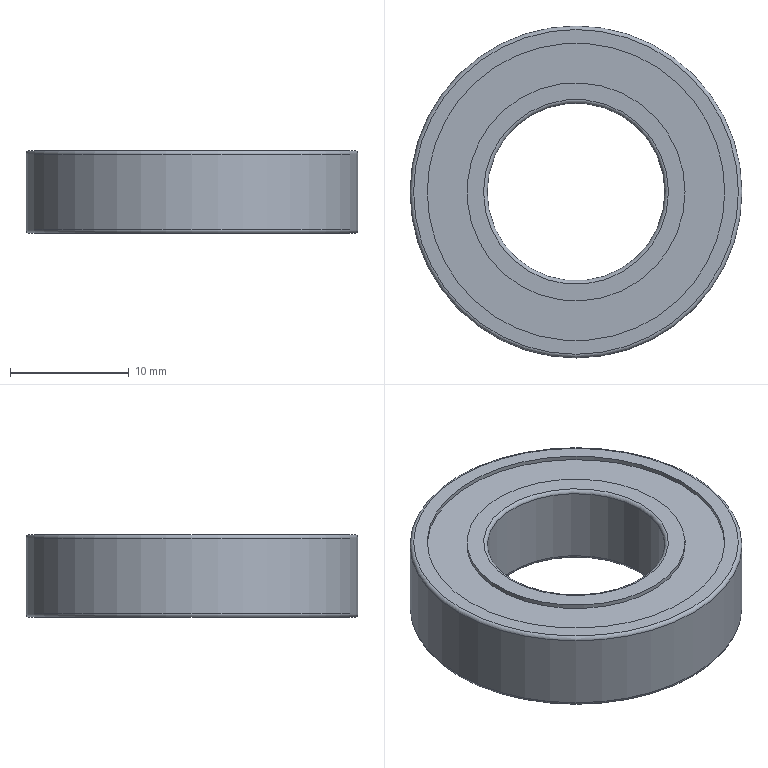Part | NX | features Bearing_5003_005_BGRB6902ZZ-25 2 | 1 solid | 16 faces | box 28 x 28 x 7 mm | volume 2908 mm3 | cylinder 6 | plane 6 | torus 4 | commonest cylinder face diameters 18.4 x2 25.1 x2 15 x1 28 x1
STEP:
#1=CARTESIAN_POINT('',(151.025,-322.,-244.55));
#2=VERTEX_POINT('',#1);
#3=CARTESIAN_POINT('',(158.525,-322.,-244.55));
#4=DIRECTION('',(0.,0.,1.));
#5=DIRECTION('',(-1.,0.,0.));
#6=AXIS2_PLACEMENT_3D('',#3,#4,#5);
#7=CIRCLE('',#6,7.5);
#8=EDGE_CURVE('',#2,#2,#7,.F.);
#9=ORIENTED_EDGE('',*,*,#8,.T.);
#10=EDGE_LOOP('',(#9));
#11=FACE_BOUND('',#10,.T.);
#12=CARTESIAN_POINT('',(166.025,-322.,-238.15));
#13=VERTEX_POINT('',#12);
#14=CARTESIAN_POINT('',(158.525,-322.,-238.15));
#15=DIRECTION('',(0.,0.,-1.));
#16=DIRECTION('',(1.,0.,0.));
#17=AXIS2_PLACEMENT_3D('',#14,#15,#16);
#18=CIRCLE('',#17,7.5);
#19=EDGE_CURVE('',#13,#13,#18,.F.);
#20=ORIENTED_EDGE('',*,*,#19,.T.);
#21=EDGE_LOOP('',(#20));
#22=FACE_BOUND('',#21,.T.);
#23=CARTESIAN_POINT('',(158.525,-322.,-244.85));
#24=DIRECTION('',(0.,0.,-1.));
#25=DIRECTION('',(1.,0.,0.));
#26=AXIS2_PLACEMENT_3D('',#23,#24,#25);
#27=CYLINDRICAL_SURFACE('',#26,7.5);
#28=ADVANCED_FACE('',(#11,#22),#27,.F.);
#29=CARTESIAN_POINT('',(150.725,-322.,-244.85));
#30=VERTEX_POINT('',#29);
#31=CARTESIAN_POINT('',(158.525,-322.,-244.85));
#32=DIRECTION('',(0.,0.,1.));
#33=DIRECTION('',(-1.,0.,0.));
#34=AXIS2_PLACEMENT_3D('',#31,#32,#33);
#35=CIRCLE('',#34,7.8);
#36=EDGE_CURVE('',#30,#30,#35,.T.);
#37=ORIENTED_EDGE('',*,*,#36,.T.);
#38=EDGE_LOOP('',(#37));
#39=FACE_BOUND('',#38,.T.);
#40=CARTESIAN_POINT('',(167.725,-322.,-244.85));
#41=VERTEX_POINT('',#40);
#42=CARTESIAN_POINT('',(158.525,-322.,-244.85));
#43=DIRECTION('',(0.,0.,-1.));
#44=DIRECTION('',(1.,0.,0.));
#45=AXIS2_PLACEMENT_3D('',#42,#43,#44);
#46=CIRCLE('',#45,9.2);
#47=EDGE_CURVE('',#41,#41,#46,.T.);
#48=ORIENTED_EDGE('',*,*,#47,.T.);
#49=EDGE_LOOP('',(#48));
#50=FACE_BOUND('',#49,.T.);
#51=CARTESIAN_POINT('',(151.025,-322.,-244.85));
#52=DIRECTION('',(0.,0.,1.));
#53=DIRECTION('',(-1.,0.,0.));
#54=AXIS2_PLACEMENT_3D('',#51,#52,#53);
#55=PLANE('',#54);
#56=ADVANCED_FACE('',(#39,#50),#55,.F.);
#57=ORIENTED_EDGE('',*,*,#47,.F.);
#58=EDGE_LOOP('',(#57));
#59=FACE_BOUND('',#58,.T.);
#60=CARTESIAN_POINT('',(167.725,-322.,-244.5));
#61=VERTEX_POINT('',#60);
#62=CARTESIAN_POINT('',(158.525,-322.,-244.5));
#63=DIRECTION('',(0.,0.,-1.));
#64=DIRECTION('',(1.,0.,0.));
#65=AXIS2_PLACEMENT_3D('',#62,#63,#64);
#66=CIRCLE('',#65,9.2);
#67=EDGE_CURVE('',#61,#61,#66,.T.);
#68=ORIENTED_EDGE('',*,*,#67,.T.);
#69=EDGE_LOOP('',(#68));
#70=FACE_BOUND('',#69,.T.);
#71=CARTESIAN_POINT('',(158.525,-322.,-244.85));
#72=DIRECTION('',(0.,0.,-1.));
#73=DIRECTION('',(1.,0.,0.));
#74=AXIS2_PLACEMENT_3D('',#71,#72,#73);
#75=CYLINDRICAL_SURFACE('',#74,9.2);
#76=ADVANCED_FACE('',(#59,#70),#75,.T.);
#77=ORIENTED_EDGE('',*,*,#67,.F.);
#78=EDGE_LOOP('',(#77));
#79=FACE_BOUND('',#78,.T.);
#80=CARTESIAN_POINT('',(171.075,-322.,-244.5));
#81=VERTEX_POINT('',#80);
#82=CARTESIAN_POINT('',(158.525,-322.,-244.5));
#83=DIRECTION('',(0.,0.,-1.));
#84=DIRECTION('',(1.,0.,0.));
#85=AXIS2_PLACEMENT_3D('',#82,#83,#84);
#86=CIRCLE('',#85,12.55);
#87=EDGE_CURVE('',#81,#81,#86,.T.);
#88=ORIENTED_EDGE('',*,*,#87,.T.);
#89=EDGE_LOOP('',(#88));
#90=FACE_BOUND('',#89,.T.);
#91=CARTESIAN_POINT('',(149.325,-322.,-244.5));
#92=DIRECTION('',(0.,0.,1.));
#93=DIRECTION('',(-1.,0.,0.));
#94=AXIS2_PLACEMENT_3D('',#91,#92,#93);
#95=PLANE('',#94);
#96=ADVANCED_FACE('',(#79,#90),#95,.F.);
#97=ORIENTED_EDGE('',*,*,#87,.F.);
#98=EDGE_LOOP('',(#97));
#99=FACE_BOUND('',#98,.T.);
#100=CARTESIAN_POINT('',(171.075,-322.,-244.85));
#101=VERTEX_POINT('',#100);
#102=CARTESIAN_POINT('',(158.525,-322.,-244.85));
#103=DIRECTION('',(0.,0.,-1.));
#104=DIRECTION('',(1.,0.,0.));
#105=AXIS2_PLACEMENT_3D('',#102,#103,#104);
#106=CIRCLE('',#105,12.55);
#107=EDGE_CURVE('',#101,#101,#106,.T.);
#108=ORIENTED_EDGE('',*,*,#107,.T.);
#109=EDGE_LOOP('',(#108));
#110=FACE_BOUND('',#109,.T.);
#111=CARTESIAN_POINT('',(158.525,-322.,-244.85));
#112=DIRECTION('',(0.,0.,-1.));
#113=DIRECTION('',(1.,0.,0.));
#114=AXIS2_PLACEMENT_3D('',#111,#112,#113);
#115=CYLINDRICAL_SURFACE('',#114,12.55);
#116=ADVANCED_FACE('',(#99,#110),#115,.F.);
#117=CARTESIAN_POINT('',(144.825,-322.,-244.85));
#118=VERTEX_POINT('',#117);
#119=CARTESIAN_POINT('',(158.525,-322.,-244.85));
#120=DIRECTION('',(0.,0.,1.));
#121=DIRECTION('',(-1.,0.,0.));
#122=AXIS2_PLACEMENT_3D('',#119,#120,#121);
#123=CIRCLE('',#122,13.7);
#124=EDGE_CURVE('',#118,#118,#123,.F.);
#125=ORIENTED_EDGE('',*,*,#124,.T.);
#126=EDGE_LOOP('',(#125));
#127=FACE_BOUND('',#126,.T.);
#128=ORIENTED_EDGE('',*,*,#107,.F.);
#129=EDGE_LOOP('',(#128));
#130=FACE_BOUND('',#129,.T.);
#131=CARTESIAN_POINT('',(145.975,-322.,-244.85));
#132=DIRECTION('',(0.,0.,1.));
#133=DIRECTION('',(-1.,0.,0.));
#134=AXIS2_PLACEMENT_3D('',#131,#132,#133);
#135=PLANE('',#134);
#136=ADVANCED_FACE('',(#127,#130),#135,.F.);
#137=CARTESIAN_POINT('',(144.525,-322.,-244.55));
#138=VERTEX_POINT('',#137);
#139=CARTESIAN_POINT('',(158.525,-322.,-244.55));
#140=DIRECTION('',(0.,0.,1.));
#141=DIRECTION('',(-1.,0.,0.));
#142=AXIS2_PLACEMENT_3D('',#139,#140,#141);
#143=CIRCLE('',#142,14.);
#144=EDGE_CURVE('',#138,#138,#143,.T.);
#145=ORIENTED_EDGE('',*,*,#144,.T.);
#146=EDGE_LOOP('',(#145));
#147=FACE_BOUND('',#146,.T.);
#148=CARTESIAN_POINT('',(172.525,-322.,-238.15));
#149=VERTEX_POINT('',#148);
#150=CARTESIAN_POINT('',(158.525,-322.,-238.15));
#151=DIRECTION('',(0.,0.,-1.));
#152=DIRECTION('',(1.,0.,0.));
#153=AXIS2_PLACEMENT_3D('',#150,#151,#152);
#154=CIRCLE('',#153,14.);
#155=EDGE_CURVE('',#149,#149,#154,.T.);
#156=ORIENTED_EDGE('',*,*,#155,.T.);
#157=EDGE_LOOP('',(#156));
#158=FACE_BOUND('',#157,.T.);
#159=CARTESIAN_POINT('',(158.525,-322.,-244.85));
#160=DIRECTION('',(0.,0.,-1.));
#161=DIRECTION('',(1.,0.,0.));
#162=AXIS2_PLACEMENT_3D('',#159,#160,#161);
#163=CYLINDRICAL_SURFACE('',#162,14.);
#164=ADVANCED_FACE('',(#147,#158),#163,.T.);
#165=CARTESIAN_POINT('',(172.225,-322.,-237.85));
#166=VERTEX_POINT('',#165);
#167=CARTESIAN_POINT('',(158.525,-322.,-237.85));
#168=DIRECTION('',(0.,0.,-1.));
#169=DIRECTION('',(1.,0.,0.));
#170=AXIS2_PLACEMENT_3D('',#167,#168,#169);
#171=CIRCLE('',#170,13.7);
#172=EDGE_CURVE('',#166,#166,#171,.F.);
#173=ORIENTED_EDGE('',*,*,#172,.T.);
#174=EDGE_LOOP('',(#173));
#175=FACE_BOUND('',#174,.T.);
#176=CARTESIAN_POINT('',(171.075,-322.,-237.85));
#177=VERTEX_POINT('',#176);
#178=CARTESIAN_POINT('',(158.525,-322.,-237.85));
#179=DIRECTION('',(0.,0.,-1.));
#180=DIRECTION('',(1.,0.,0.));
#181=AXIS2_PLACEMENT_3D('',#178,#179,#180);
#182=CIRCLE('',#181,12.55);
#183=EDGE_CURVE('',#177,#177,#182,.T.);
#184=ORIENTED_EDGE('',*,*,#183,.T.);
#185=EDGE_LOOP('',(#184));
#186=FACE_BOUND('',#185,.T.);
#187=CARTESIAN_POINT('',(144.525,-322.,-237.85));
#188=DIRECTION('',(0.,0.,-1.));
#189=DIRECTION('',(1.,0.,0.));
#190=AXIS2_PLACEMENT_3D('',#187,#188,#189);
#191=PLANE('',#190);
#192=ADVANCED_FACE('',(#175,#186),#191,.F.);
#193=ORIENTED_EDGE('',*,*,#183,.F.);
#194=EDGE_LOOP('',(#193));
#195=FACE_BOUND('',#194,.T.);
#196=CARTESIAN_POINT('',(171.075,-322.,-238.2));
#197=VERTEX_POINT('',#196);
#198=CARTESIAN_POINT('',(158.525,-322.,-238.2));
#199=DIRECTION('',(0.,0.,-1.));
#200=DIRECTION('',(1.,0.,0.));
#201=AXIS2_PLACEMENT_3D('',#198,#199,#200);
#202=CIRCLE('',#201,12.55);
#203=EDGE_CURVE('',#197,#197,#202,.T.);
#204=ORIENTED_EDGE('',*,*,#203,.T.);
#205=EDGE_LOOP('',(#204));
#206=FACE_BOUND('',#205,.T.);
#207=CARTESIAN_POINT('',(158.525,-322.,-244.85));
#208=DIRECTION('',(0.,0.,-1.));
#209=DIRECTION('',(1.,0.,0.));
#210=AXIS2_PLACEMENT_3D('',#207,#208,#209);
#211=CYLINDRICAL_SURFACE('',#210,12.55);
#212=ADVANCED_FACE('',(#195,#206),#211,.F.);
#213=ORIENTED_EDGE('',*,*,#203,.F.);
#214=EDGE_LOOP('',(#213));
#215=FACE_BOUND('',#214,.T.);
#216=CARTESIAN_POINT('',(167.725,-322.,-238.2));
#217=VERTEX_POINT('',#216);
#218=CARTESIAN_POINT('',(158.525,-322.,-238.2));
#219=DIRECTION('',(0.,0.,-1.));
#220=DIRECTION('',(1.,0.,0.));
#221=AXIS2_PLACEMENT_3D('',#218,#219,#220);
#222=CIRCLE('',#221,9.2);
#223=EDGE_CURVE('',#217,#217,#222,.T.);
#224=ORIENTED_EDGE('',*,*,#223,.T.);
#225=EDGE_LOOP('',(#224));
#226=FACE_BOUND('',#225,.T.);
#227=CARTESIAN_POINT('',(145.975,-322.,-238.2));
#228=DIRECTION('',(0.,0.,-1.));
#229=DIRECTION('',(1.,0.,0.));
#230=AXIS2_PLACEMENT_3D('',#227,#228,#229);
#231=PLANE('',#230);
#232=ADVANCED_FACE('',(#215,#226),#231,.F.);
#233=ORIENTED_EDGE('',*,*,#223,.F.);
#234=EDGE_LOOP('',(#233));
#235=FACE_BOUND('',#234,.T.);
#236=CARTESIAN_POINT('',(167.725,-322.,-237.85));
#237=VERTEX_POINT('',#236);
#238=CARTESIAN_POINT('',(158.525,-322.,-237.85));
#239=DIRECTION('',(0.,0.,-1.));
#240=DIRECTION('',(1.,0.,0.));
#241=AXIS2_PLACEMENT_3D('',#238,#239,#240);
#242=CIRCLE('',#241,9.2);
#243=EDGE_CURVE('',#237,#237,#242,.T.);
#244=ORIENTED_EDGE('',*,*,#243,.T.);
#245=EDGE_LOOP('',(#244));
#246=FACE_BOUND('',#245,.T.);
#247=CARTESIAN_POINT('',(158.525,-322.,-244.85));
#248=DIRECTION('',(0.,0.,-1.));
#249=DIRECTION('',(1.,0.,0.));
#250=AXIS2_PLACEMENT_3D('',#247,#248,#249);
#251=CYLINDRICAL_SURFACE('',#250,9.2);
#252=ADVANCED_FACE('',(#235,#246),#251,.T.);
#253=CARTESIAN_POINT('',(166.325,-322.,-237.85));
#254=VERTEX_POINT('',#253);
#255=CARTESIAN_POINT('',(158.525,-322.,-237.85));
#256=DIRECTION('',(0.,0.,-1.));
#257=DIRECTION('',(1.,0.,0.));
#258=AXIS2_PLACEMENT_3D('',#255,#256,#257);
#259=CIRCLE('',#258,7.8);
#260=EDGE_CURVE('',#254,#254,#259,.T.);
#261=ORIENTED_EDGE('',*,*,#260,.T.);
#262=EDGE_LOOP('',(#261));
#263=FACE_BOUND('',#262,.T.);
#264=ORIENTED_EDGE('',*,*,#243,.F.);
#265=EDGE_LOOP('',(#264));
#266=FACE_BOUND('',#265,.T.);
#267=CARTESIAN_POINT('',(149.325,-322.,-237.85));
#268=DIRECTION('',(0.,0.,-1.));
#269=DIRECTION('',(1.,0.,0.));
#270=AXIS2_PLACEMENT_3D('',#267,#268,#269);
#271=PLANE('',#270);
#272=ADVANCED_FACE('',(#263,#266),#271,.F.);
#273=ORIENTED_EDGE('',*,*,#36,.F.);
#274=EDGE_LOOP('',(#273));
#275=FACE_BOUND('',#274,.T.);
#276=ORIENTED_EDGE('',*,*,#8,.F.);
#277=EDGE_LOOP('',(#276));
#278=FACE_BOUND('',#277,.T.);
#279=CARTESIAN_POINT('',(158.525,-322.,-244.55));
#280=DIRECTION('',(0.,0.,1.));
#281=DIRECTION('',(-1.,0.,0.));
#282=AXIS2_PLACEMENT_3D('',#279,#280,#281);
#283=TOROIDAL_SURFACE('',#282,7.8,0.3);
#284=ADVANCED_FACE('',(#275,#278),#283,.T.);
#285=ORIENTED_EDGE('',*,*,#19,.F.);
#286=EDGE_LOOP('',(#285));
#287=FACE_BOUND('',#286,.T.);
#288=ORIENTED_EDGE('',*,*,#260,.F.);
#289=EDGE_LOOP('',(#288));
#290=FACE_BOUND('',#289,.T.);
#291=CARTESIAN_POINT('',(158.525,-322.,-238.15));
#292=DIRECTION('',(0.,0.,-1.));
#293=DIRECTION('',(1.,0.,0.));
#294=AXIS2_PLACEMENT_3D('',#291,#292,#293);
#295=TOROIDAL_SURFACE('',#294,7.8,0.3);
#296=ADVANCED_FACE('',(#287,#290),#295,.T.);
#297=ORIENTED_EDGE('',*,*,#144,.F.);
#298=EDGE_LOOP('',(#297));
#299=FACE_BOUND('',#298,.T.);
#300=ORIENTED_EDGE('',*,*,#124,.F.);
#301=EDGE_LOOP('',(#300));
#302=FACE_BOUND('',#301,.T.);
#303=CARTESIAN_POINT('',(158.525,-322.,-244.55));
#304=DIRECTION('',(0.,0.,1.));
#305=DIRECTION('',(-1.,0.,0.));
#306=AXIS2_PLACEMENT_3D('',#303,#304,#305);
#307=TOROIDAL_SURFACE('',#306,13.7,0.3);
#308=ADVANCED_FACE('',(#299,#302),#307,.T.);
#309=ORIENTED_EDGE('',*,*,#172,.F.);
#310=EDGE_LOOP('',(#309));
#311=FACE_BOUND('',#310,.T.);
#312=ORIENTED_EDGE('',*,*,#155,.F.);
#313=EDGE_LOOP('',(#312));
#314=FACE_BOUND('',#313,.T.);
#315=CARTESIAN_POINT('',(158.525,-322.,-238.15));
#316=DIRECTION('',(0.,0.,-1.));
#317=DIRECTION('',(1.,0.,0.));
#318=AXIS2_PLACEMENT_3D('',#315,#316,#317);
#319=TOROIDAL_SURFACE('',#318,13.7,0.3);
#320=ADVANCED_FACE('',(#311,#314),#319,.T.);
#321=CLOSED_SHELL('',(#28,#56,#76,#96,#116,#136,#164,#192,#212,#232,#252,#272,#284,#296,#308,#320));
#322=MANIFOLD_SOLID_BREP('',#321);
#323=(LENGTH_UNIT()NAMED_UNIT(*)SI_UNIT(.MILLI.,.METRE.));
#324=UNCERTAINTY_MEASURE_WITH_UNIT(LENGTH_MEASURE(0.00001),#323,'','');
#325=(NAMED_UNIT(*)PLANE_ANGLE_UNIT()SI_UNIT($,.RADIAN.));
#326=(NAMED_UNIT(*)SI_UNIT($,.STERADIAN.)SOLID_ANGLE_UNIT());
#327=(GEOMETRIC_REPRESENTATION_CONTEXT(3)GLOBAL_UNCERTAINTY_ASSIGNED_CONTEXT((#324))GLOBAL_UNIT_ASSIGNED_CONTEXT((#323,#325,#326))REPRESENTATION_CONTEXT('',''));
#328=ADVANCED_BREP_SHAPE_REPRESENTATION('',(#322),#327);